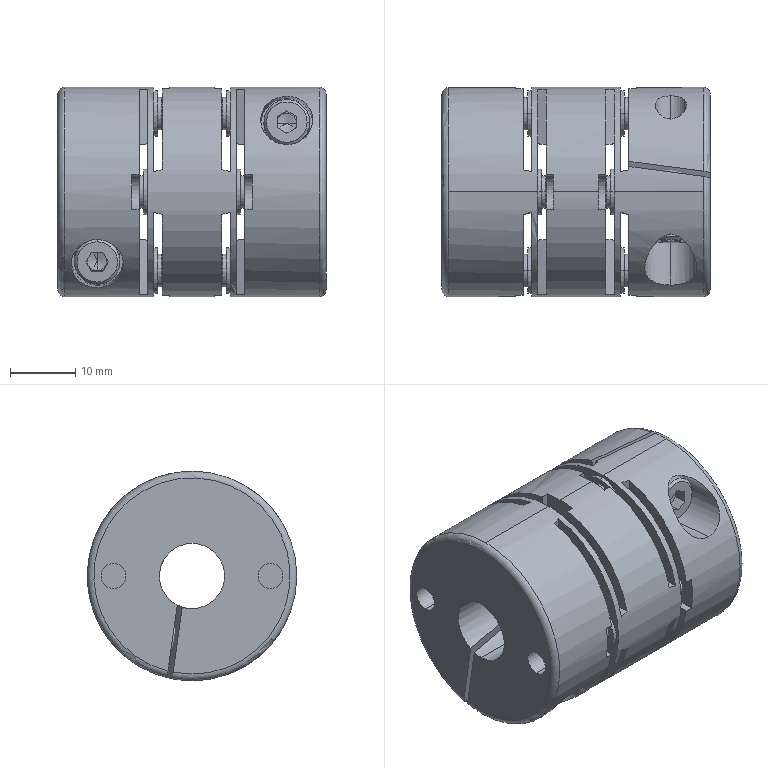Part | SolidWorks | 3 solids | 224 faces | box 41 x 32 x 32 mm | volume 23844 mm3 | plane 105 | cylinder 97 | cone 20 | torus 2 | commonest cylinder face diameters 7 x20 5 x16 3.8 x8 4 x8 5.4 x8 16 x8